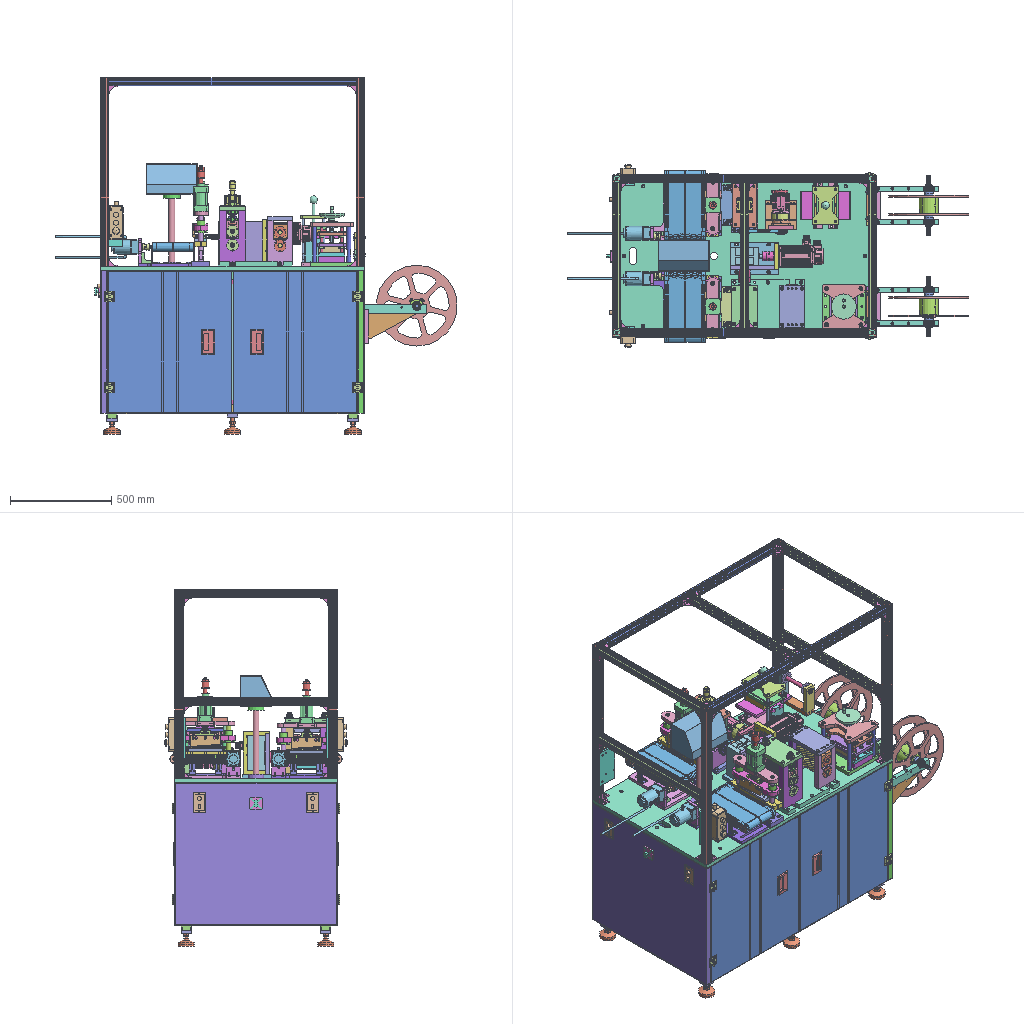Assembly | STEP file | 152 different items | 378 placed | box 1984 x 906 x 1760 mm
Parts list (item | name | quantity | parent item | size | volume):
1 | YBQDJ-FLJ-1 | x4 | in YBQDJ-FLJ | 400 x 8 x 400 mm | 566908 mm3
2 | YBQDJ-FLJ-3 | x2 | in YBQDJ-FLJ | - | -
3 | YBQDJ-FLJ-2 | x2 | in YBQDJ-FLJ | 95 x 103 x 95 mm | 482469 mm3
4 | YBQDJ-FLJ-5 | x2 | in YBQDJ-FLJ | 20 x 190 x 190 mm | 661776 mm3
5 | YBQDJ-FLJ-4 | x4 | in YBQDJ-FLJ | 310 x 25 x 45 mm | 300462 mm3
6 | YBQDJ-FLJ-6 | x4 | in YBQDJ-FLJ | 237.857 x 15 x 120 mm | 224363 mm3
7 | YBQDJ-FLJ-7 | x8 | in YBQDJ-FLJ | 15 x 33 x 33 mm | 11378 mm3
8 | YBQDJ-YL-1 | x1 | in YBQDJ-YL | 210 x 210 x 20 mm | 848713 mm3
9 | YBQDJ-YL-8 | x4 | in YBQDJ-YL | 12 x 12 x 182 mm | 19664 mm3
10 | YBQDJ-YL-13 | x2 | in YBQDJ-YL | 18.475 x 16 x 75 mm | 8074 mm3
11 | YBQDJ-YL-2 | x2 | in YBQDJ-YL | 130 x 30 x 30 mm | 104775 mm3
12 | YBQDJ-YL-10 | x1 | in YBQDJ-YL | 125 x 125 x 70 mm | 226936 mm3
13 | YBQDJ-YL-5 | x1 | in YBQDJ-YL | 140 x 220 x 15 mm | 360572 mm3
14 | YBQDJ-YL-9 | x4 | in YBQDJ-YL | 20 x 20 x 198 mm | 57396 mm3
15 | YBQDJ-YL-14 | x8 | in YBQDJ-YL | 32 x 32 x 30 mm | 10494 mm3
16 | YBQDJ-YL-12 | x1 | in YBQDJ-YL | 24.249 x 21 x 7 mm | 1795 mm3
17 | YBQDJ-YL-3 | x1 | in YBQDJ-YL | 130 x 210 x 15 mm | 393827 mm3
18 | YBQDJ-YL-7 | x1 | in YBQDJ-YL | 130 x 120 x 30 mm | 464984 mm3
19 | YBQDJ-YL-4 | x1 | in YBQDJ-YL | 140 x 220 x 15 mm | 408740 mm3
20 | YBQDJ-YL-11 | x1 | in YBQDJ-YL | 20 x 20 x 118 mm | 24858 mm3
21 | YBQDJ-YL-6 | x1 | in YBQDJ-YL | 210 x 220 x 20 mm | 625567 mm3
22 | YBQDJ-YL-15 | x2 | in YBQDJ-YL | 54 x 54 x 6 mm | 8414 mm3
23 | YBQDJ-YL-16 | x2 | in YBQDJ-YL | 32 x 32 x 9 mm | 3911 mm3
24 | YBQDJ-YL-17 | x1 | in YBQDJ-YL | 44 x 44 x 32 mm | 13018 mm3
25 | YBQDJ-YB-1 | x1 | in YBQDJ-YB | 360 x 270 x 24 mm | 2084097 mm3
26 | YBQDJ-YB-3 | x2 | in YBQDJ-YB | 80 x 30 x 70 mm | 107518 mm3
27 | YBQDJ-YB-18 | x1 | in YBQDJ-YB | 220 x 20 x 210 mm | 773333 mm3
28 | YBQDJ-YB-16 | x1 | in YBQDJ-YB | 33 x 210 x 33 mm | 88192 mm3
29 | YBQDJ-YB-17 | x1 | in YBQDJ-YB | 55 x 66 x 55 mm | 122440 mm3
30 | YBQDJ-YB-20 | x1 | in YBQDJ-YB | 193 x 155 x 174 mm | 2083887 mm3
31 | YBQDJ-YB-5 | x2 | in YBQDJ-YB | 68.992 x 218 x 68.953 mm | 543044 mm3
32 | YBQDJ-YB-6 | x1 | in YBQDJ-YB | 130 x 38 x 273 mm | 843391 mm3
33 | YBQDJ-YB-15 | x2 | in YBQDJ-YB | 69.832 x 130 x 69.818 mm | 396551 mm3
34 | YBQDJ-YB-8 | x2 | in YBQDJ-YB | 30 x 34.641 x 119.5 mm | 39653 mm3
35 | YBQDJ-YB-13 | x2 | in YBQDJ-YB | 59 x 10.5 x 59 mm | 15659 mm3
36 | YBQDJ-YB-12 | x2 | in YBQDJ-YB | 59 x 19 x 59 mm | 24092 mm3
37 | YBQDJ-YB-22 | x1 | in YBQDJ-YB | 275 x 158 x 110 mm | 3118501 mm3
38 | YBQDJ-YB-9 | x4 | in YBQDJ-YB | 50 x 50 x 14 mm | 18346 mm3
39 | YBQDJ-YB-7 | x2 | in YBQDJ-YB | 76 x 38 x 80 mm | 112101 mm3
40 | YBQDJ-YB-19 | x1 | in YBQDJ-YB | 240 x 160 x 19 mm | 686478 mm3
41 | YBQDJ-YB-21 | x1 | in YBQDJ-YB | 20 x 130 x 210 mm | 393461 mm3
42 | YBQDJ-YB-2 | x1 | in YBQDJ-YB | 120 x 30 x 223 mm | 466414 mm3
43 | YBQDJ-YB-11 | x1 | in YBQDJ-YB | 33 x 245 x 33 mm | 98573 mm3
44 | YBQDJ-YB-14 | x4 | in YBQDJ-YB | 59 x 5 x 59 mm | 11475 mm3
45 | YBQDJ-YB-4 | x1 | in YBQDJ-YB | 120 x 210 x 20 mm | 483124 mm3
46 | YBQDJ-YB-10 | x2 | in YBQDJ-YB | 42.8 x 42.8 x 20 mm | 13331 mm3
47 | YBQDJ-YB-23 | x1 | in YBQDJ-YB | 55 x 45 x 45 mm | 72571 mm3
48 | YBQDJ-YB-24 | x2 | in YBQDJ-YB | 30 x 10 x 30 mm | 3895 mm3
49 | YBQDJ-YB-25 | x1 | in YBQDJ-YB | - | -
50 | YBQDJ-YB-27 | x1 | in YBQDJ-YB | 130 x 38 x 273 mm | 843391 mm3
51 | YBQDJ-YB-26 | x1 | in YBQDJ-YB | 120 x 30 x 223 mm | 466414 mm3
52 | YBQDJ-YB-28 | x1 | in YBQDJ-YB | 130 x 210 x 20 mm | 518119 mm3
53 | YBQDJ-YB-29 | x16 | in YBQDJ-YB | 42 x 12 x 42 mm | 8686 mm3
54 | YBQDJ-YB-30 | x2 | in YBQDJ-YB | 34.5 x 10 x 4 mm | 1380 mm3
55 | YBQDJ-YB-34 | x1 | in YBQDJ-YB | 164.076 x 196 x 5.026 mm | 23129 mm3
56 | YBQDJ-YB-31 | x2 | in YBQDJ-YB | 40 x 30 x 80 mm | 9225 mm3
57 | YBQDJ-YB-32 | x1 | in YBQDJ-YB | 139.076 x 196 x 5.026 mm | 26086 mm3
58 | YBQDJ-YB-33 | x2 | in YBQDJ-YB | 20 x 20 x 4 mm | 942.478 mm3
59 | YBQDJ-QD-1 | x2 | in YBQDJ-QD-BD, YBQDJ-QD-PD | 90 x 300 x 25 mm | 495978 mm3
60 | YBQDJ-QD-7 | x4 | in YBQDJ-QD-BD, YBQDJ-QD-PD | 62 x 62 x 59 mm | 57722 mm3
61 | YBQDJ-QD-10 | x2 | in YBQDJ-QD-BD, YBQDJ-QD-PD | 75 x 290 x 20 mm | 318824 mm3
62 | YBQDJ-QD-4 | x2 | in YBQDJ-QD-BD, YBQDJ-QD-PD | 20 x 190 x 15 mm | 51822 mm3
63 | YBQDJ-QD-3 | x2 | in YBQDJ-QD-BD, YBQDJ-QD-PD | 60 x 310 x 25 mm | 397510 mm3
64 | YBQDJ-QD-2 | x2 | in YBQDJ-QD-BD | 25 x 25 x 254 mm | 111454 mm3
65 | YBQDJ-QD-11 | x2 | in YBQDJ-QD-BD, YBQDJ-QD-PD | 75 x 75 x 272 mm | 699847 mm3
66 | YBQDJ-QD-5 | x2 | in YBQDJ-QD-BD, YBQDJ-QD-PD | 35 x 190 x 15 mm | 92776 mm3
67 | YBQDJ-QD-8 | x2 | in YBQDJ-QD-BD, YBQDJ-QD-PD | 35 x 90 x 25 mm | 38677 mm3
68 | YBQDJ-QD-6 | x2 | in YBQDJ-QD-BD, YBQDJ-QD-PD | 70 x 300 x 25 mm | 414235 mm3
69 | YBQDJ-QD-9 | x2 | in YBQDJ-QD-BD, YBQDJ-QD-PD | 34 x 34 x 24 mm | 13509 mm3
70 | YBQDJ-QD-12 | x2 | in YBQDJ-QD-BD, YBQDJ-QD-PD | 10 x 150 x 65 mm | 69081 mm3
71 | YBQDJ-SSJ-1 | x1 | in YBQDJ-SSJ-BD | 280 x 320 x 15 mm | 982860 mm3
72 | YBQDJ-SSJ-8 | x2 | in YBQDJ-SSJ-BD, YBQD-SSJ-PD_MODEL | 50 x 20 x 50 mm | 24742 mm3
73 | YBQDJ-SSJ-7 | x2 | in YBQDJ-SSJ-BD, YBQD-SSJ-PD_MODEL | 227 x 40.957 x 41.285 mm | 212732 mm3
74 | YBQDJ-SSJ-3 | x2 | in YBQDJ-SSJ-BD, YBQD-SSJ-PD_MODEL | 200 x 350 x 44 mm | 311989 mm3
75 | YBQDJ-SSJ-11 | x2 | in YBQDJ-SSJ-BD, YBQD-SSJ-PD_MODEL | 35 x 30 x 30 mm | 20965 mm3
76 | YBQDJ-SSJ-9 | x2 | in YBQDJ-SSJ-BD, YBQD-SSJ-PD_MODEL | 15 x 70 x 120 mm | 105388 mm3
77 | YBQDJ-SSJ-6 | x2 | in YBQDJ-SSJ-BD, YBQD-SSJ-PD_MODEL | 196 x 40 x 40 mm | 211425 mm3
78 | YBQDJ-SSJ-4 | x8 | in YBQDJ-SSJ-BD, YBQD-SSJ-PD_MODEL | 20 x 85 x 39 mm | 27065 mm3
79 | YBQDJ-SSJ-10 | x2 | in YBQDJ-SSJ-BD, YBQD-SSJ-PD_MODEL | - | -
80 | YBQDJ-SSJ-2 | x8 | in YBQDJ-SSJ-BD, YBQD-SSJ-PD_MODEL | 40 x 30 x 80 mm | 9225 mm3
81 | YBQDJ-SSJ-5 | x4 | in YBQDJ-SSJ-BD, YBQD-SSJ-PD_MODEL | 20 x 215 x 40 mm | 63524 mm3
82 | YBQDJ-YY-1 | x1 | in YBQDJ-YY | 120 x 230 x 20 mm | 476492 mm3
83 | YBQDJ-YY-3 | x1 | in YBQDJ-YY | 80 x 20 x 148 mm | 197857 mm3
84 | YBQDJ-YY-5 | x1 | in YBQDJ-YY | 130 x 120 x 30 mm | 465920 mm3
85 | YBQDJ-YY-2 | x1 | in YBQDJ-YY | 80 x 20 x 148 mm | 197857 mm3
86 | YBQDJ-YY-7 | x1 | in YBQDJ-YY | 130 x 190 x 15 mm | 325427 mm3
87 | YBQDJ-YY-6 | x4 | in YBQDJ-YY | 32 x 32 x 30 mm | 10494 mm3
88 | YBQDJ-YY-10 | x4 | in YBQDJ-YY | 12 x 12 x 237 mm | 24995 mm3
89 | YBQDJ-YY-8 | x1 | in YBQDJ-YY | 130 x 190 x 15 mm | 272574 mm3
90 | YBQDJ-YY-4 | x1 | in YBQDJ-YY | 250 x 190 x 15 mm | 563148 mm3
91 | YBQDJ-YY-9 | x1 | in YBQDJ-YY | 40 x 40 x 166 mm | 52339 mm3
92 | YBQDJ-PD-1 | x1 | in YBQDJ-PD_MODEL | 150 x 140 x 20 mm | 385255 mm3
93 | YBQDJ-PD-4 | x2 | in YBQDJ-PD_MODEL | 67 x 28.5 x 67 mm | 55543 mm3
94 | YBQDJ-PD-7 | x1 | in YBQDJ-PD_MODEL | 130 x 29.2 x 127.5 mm | 362195 mm3
95 | YBQDJ-PD-3 | x1 | in YBQDJ-PD_MODEL | 120 x 20 x 138 mm | 191169 mm3
96 | YBQDJ-PD-5 | x1 | in YBQDJ-PD_MODEL | 245.482 x 15 x 95 mm | 17074 mm3
97 | YBQDJ-PD-9 | x1 | in YBQDJ-PD_MODEL | 68.992 x 253 x 68.953 mm | 537694 mm3
98 | YBQDJ-PD-8 | x1 | in YBQDJ-PD_MODEL | 130 x 29.2 x 127.5 mm | 362195 mm3
99 | YBQDJ-PD-11 | x4 | in YBQDJ-PD_MODEL | 32 x 32 x 57 mm | 16408 mm3
100 | YBQDJ-PD-10 | x1 | in YBQDJ-PD_MODEL | 68.992 x 218 x 68.953 mm | 532441 mm3
101 | YBQDJ-PD-6 | x1 | in YBQDJ-PD_MODEL | 130 x 270 x 19 mm | 640127 mm3
102 | YBQDJ-PD-2 | x1 | in YBQDJ-PD_MODEL | - | 675014 mm3
103 | YBQDJ-PD-16 | x1 | in YBQDJ-PD_MODEL | 34 x 34 x 24 mm | 12336 mm3
104 | YBQDJ-PD-15 | x1 | in YBQDJ-PD_MODEL | 76 x 84.5 x 162 mm | 333527 mm3
105 | YBQDJ-PD-17 | x1 | in YBQDJ-PD_MODEL | 35 x 90 x 25 mm | 38677 mm3
106 | YBQDJ-PD-13 | x4 | in YBQDJ-PD_MODEL | 12 x 12 x 284 mm | 30280 mm3
107 | YBQDJ-PD-14 | x1 | in YBQDJ-PD_MODEL | 120 x 220 x 20 mm | 489101 mm3
108 | YBQDJ-PD-18 | x1 | in YBQDJ-PD_MODEL | 40 x 220 x 15 mm | 117739 mm3
109 | YBQDJ-PD-19 | x4 | in YBQDJ-PD_MODEL | 53 x 13 x 53 mm | 13997 mm3
110 | YBQDJ-PD-12 | x2 | in YBQDJ-PD_MODEL | 130 x 29.2 x 80 mm | 97793 mm3
111 | YBQDJ-PD-20 | x8 | in YBQDJ-PD_MODEL | 35 x 11 x 35 mm | 5907 mm3
112 | YBQDJ-PD-21 | x1 | in YBQDJ-PD_MODEL | 31.177 x 27 x 9 mm | 3802 mm3
113 | YBQDJ-PD-24 | x2 | in YBQDJ-PD_MODEL | 20 x 20 x 4 mm | 1030 mm3
114 | YBQDJ-PD-25 | x2 | in YBQDJ-PD_MODEL | 40 x 30 x 80 mm | 9225 mm3
115 | YBQDJ-PD-22 | x1 | in YBQDJ-PD_MODEL | 139.076 x 196 x 5.026 mm | 26086 mm3
116 | YBQDJ-PD-23 | x1 | in YBQDJ-PD_MODEL | 164.076 x 196 x 5.026 mm | 23129 mm3
117 | YBQDJ-QD-PD-2 | x2 | in YBQDJ-QD-PD | 25 x 25 x 264 mm | 116363 mm3
118 | YBQDJ-SSJ-PD-1 | x1 | in YBQD-SSJ-PD_MODEL | 280 x 320 x 15 mm | 982860 mm3
119 | YBQDJ large plate | x1 | in Crimp-cut integrated machine, general type | 1300 x 800 x 20 mm | 20508106 mm3
120 | YBQDJ-DX-1 | x2 | in YBQDJ-DX-PD_MODEL, YBQDJ-DX-BD_MODEL | 50 x 200 x 20 mm | 177964 mm3
121 | YBQDJ-DX-3 | x4 | in YBQDJ-DX-PD_MODEL, YBQDJ-DX-BD_MODEL | 60 x 16 x 60 mm | 19587 mm3
122 | YBQDJ-DX-6 | x8 | in YBQDJ-DX-PD_MODEL, YBQDJ-DX-BD_MODEL | 32 x 10 x 32 mm | 4745 mm3
123 | YBQDJ-DX-4 | x2 | in YBQDJ-DX-PD_MODEL, YBQDJ-DX-BD_MODEL | 20 x 200 x 20 mm | 54352 mm3
124 | YBQDJ-DX-5 | x2 | in YBQDJ-DX-PD_MODEL, YBQDJ-DX-BD_MODEL | - | -
125 | YBQDJ-DX-2 | x1 | in YBQDJ-DX-PD_MODEL | 50 x 20 x 164 mm | 134384 mm3
126 | YBQDJ-DX-7 | x1 | in YBQDJ-DX-PD_MODEL | 50 x 20 x 164 mm | 134384 mm3
127 | YBQDJ-DX-BD-2 | x1 | in YBQDJ-DX-BD_MODEL | 50 x 20 x 79 mm | 49384 mm3
128 | YBQDJ-DX-BD-7 | x1 | in YBQDJ-DX-BD_MODEL | 50 x 20 x 79 mm | 49384 mm3
129 | 40x40-930 | x4 | in YBQDJ-LXC_MODEL | 40 x 40 x 930 mm | 513720 mm3
130 | 40x40-1220 | x2 | in YBQDJ-LXC_MODEL | 1220 x 40 x 40 mm | 673913 mm3
131 | 40x40-720 | x5 | in YBQDJ-LXC_MODEL | 40 x 720 x 40 mm | 397719 mm3
132 | 40x40 angle bracket | x28 | in YBQDJ-LXC_MODEL | 39.8 x 40 x 39.8 mm | 14360 mm3
133 | Button box plate | x2 | in YBQDJ-LXC_MODEL | 105 x 10 x 200 mm | 208063 mm3
134 | Button box | x2 | in YBQDJ-LXC_MODEL | 70 x 93 x 188 mm | 866675 mm3
135 | Touch screen assembly | x1 | in Crimp-cut integrated machine, general type | 250 x 150 x 505 mm | 675168 mm3
136 | 50x50x640 | x6 | in YBQDJ-JJ_MODEL | 50 x 640 x 50 mm | 562265 mm3
137 | 50x50x1240 | x2 | in YBQDJ-JJ_MODEL | 1240 x 50 x 50 mm | 1089389 mm3
138 | Foot cup | x6 | in 50x50x680_MODEL, 50x50x1140_MODEL | 80 x 80 x 135 mm | 154518 mm3
139 | Spacer block | x6 | in 50x50x680_MODEL, 50x50x1140_MODEL | 50 x 50 x 15 mm | 35145 mm3
140 | SOLID | x4 | in 50x50x680_MODEL | 50 x 50 x 680 mm | 597407 mm3
141 | Door magnet catch | x4 | in 50x50x610_MODEL | 40 x 5 x 20 mm | 3632 mm3
142 | SOLID | x2 | in 50x50x610_MODEL | 50 x 50 x 610 mm | 535909 mm3
143 | SOLID | x2 | in 50x50x1140_MODEL | 1140 x 50 x 50 mm | 1000530 mm3
144 | Crossbeam | x2 | in YBQDJ-JJ_MODEL | 15 x 730 x 50 mm | 541334 mm3
145 | Reinforcing rib | x4 | in YBQDJ-BJ-1_MODEL | 80 x 26.7 x 696 mm | 106400 mm3
146 | Handle | x4 | in YBQDJ-BJ-1_MODEL | 69 x 21 x 119 mm | 44051 mm3
147 | SOLID | x4 | in YBQDJ-BJ-1_MODEL | 615 x 30 x 705 mm | 627775 mm3
148 | Hinge | x8 | in YBQDJ-BJ_MODEL | 50 x 12.7 x 49.8 mm | 17221 mm3
149 | Power switch | x1 | in YBQDJ-BJ-2_MODEL | 64 x 60 x 60 mm | 180692 mm3
150 | Speed control panel | x2 | in YBQDJ-BJ-2_MODEL | 122.5 x 60 x 100 mm | 404808 mm3
151 | SOLID | x1 | in YBQDJ-BJ-2_MODEL | 55 x 800 x 705 mm | 825706 mm3
152 | YBQDJ-BJ-3 | x1 | in YBQDJ-BJ_MODEL | 55 x 800 x 705 mm | 823970 mm3
Placements (level | parent | child | x y z in mm | rotation matrix by rows), first 330 of 406 lines:
1 | Crimp-cut integrated machine, general type | YBQDJ-FLJ | 0.0 0.0 0.0 | 1 0 0 0 1 0 0 0 1
2 | YBQDJ-FLJ | YBQDJ-FLJ-1 | 0.0 0.0 0.0 | 1 0 0 0 1 0 0 0 1
2 | YBQDJ-FLJ | YBQDJ-FLJ-3 | 0.0 0.0 0.0 | 1 0 0 0 1 0 0 0 1
2 | YBQDJ-FLJ | YBQDJ-FLJ-2 | 0.0 0.0 0.0 | 1 0 0 0 1 0 0 0 1
2 | YBQDJ-FLJ | YBQDJ-FLJ-1 | 0.0 91.0 0.0 | 1 0 0 0 1 0 0 0 1
2 | YBQDJ-FLJ | YBQDJ-FLJ-5 | 0.0 0.0 0.0 | 1 0 0 0 1 0 0 0 1
2 | YBQDJ-FLJ | YBQDJ-FLJ-4 | 0.0 0.0 0.0 | 1 0 0 0 1 0 0 0 1
2 | YBQDJ-FLJ | YBQDJ-FLJ-6 | 0.0 0.0 0.0 | 1 0 0 0 1 0 0 0 1
2 | YBQDJ-FLJ | YBQDJ-FLJ-6 | 0.0 165.0 0.0 | 1 0 0 0 1 0 0 0 1
2 | YBQDJ-FLJ | YBQDJ-FLJ-4 | 0.0 165.0 0.0 | 1 0 0 0 1 0 0 0 1
2 | YBQDJ-FLJ | YBQDJ-FLJ-7 | -0.0 90.0 -140.0 | 1 0 0 0 1 0 0 0 1
2 | YBQDJ-FLJ | YBQDJ-FLJ-7 | -0.0 90.0 -0.0 | 1 0 0 0 1 0 0 0 1
2 | YBQDJ-FLJ | YBQDJ-FLJ-7 | 0.0 0.0 0.0 | 1 0 0 0 1 0 0 0 1
2 | YBQDJ-FLJ | YBQDJ-FLJ-7 | 0.0 0.0 -140.0 | 1 0 0 0 1 0 0 0 1
1 | Crimp-cut integrated machine, general type | YBQDJ-FLJ | 0.0 500.0 0.0 | 1 0 0 0 1 0 0 0 1
2 | YBQDJ-FLJ | YBQDJ-FLJ-1 | 0.0 0.0 0.0 | 1 0 0 0 1 0 0 0 1
2 | YBQDJ-FLJ | YBQDJ-FLJ-3 | 0.0 0.0 0.0 | 1 0 0 0 1 0 0 0 1
2 | YBQDJ-FLJ | YBQDJ-FLJ-2 | 0.0 0.0 0.0 | 1 0 0 0 1 0 0 0 1
2 | YBQDJ-FLJ | YBQDJ-FLJ-1 | 0.0 91.0 0.0 | 1 0 0 0 1 0 0 0 1
2 | YBQDJ-FLJ | YBQDJ-FLJ-5 | 0.0 0.0 0.0 | 1 0 0 0 1 0 0 0 1
2 | YBQDJ-FLJ | YBQDJ-FLJ-4 | 0.0 0.0 0.0 | 1 0 0 0 1 0 0 0 1
2 | YBQDJ-FLJ | YBQDJ-FLJ-6 | 0.0 0.0 0.0 | 1 0 0 0 1 0 0 0 1
2 | YBQDJ-FLJ | YBQDJ-FLJ-6 | 0.0 165.0 0.0 | 1 0 0 0 1 0 0 0 1
2 | YBQDJ-FLJ | YBQDJ-FLJ-4 | 0.0 165.0 0.0 | 1 0 0 0 1 0 0 0 1
2 | YBQDJ-FLJ | YBQDJ-FLJ-7 | -0.0 90.0 -140.0 | 1 0 0 0 1 0 0 0 1
2 | YBQDJ-FLJ | YBQDJ-FLJ-7 | -0.0 90.0 -0.0 | 1 0 0 0 1 0 0 0 1
2 | YBQDJ-FLJ | YBQDJ-FLJ-7 | 0.0 0.0 0.0 | 1 0 0 0 1 0 0 0 1
2 | YBQDJ-FLJ | YBQDJ-FLJ-7 | 0.0 0.0 -140.0 | 1 0 0 0 1 0 0 0 1
1 | Crimp-cut integrated machine, general type | YBQDJ-YL | 0.0 0.0 0.0 | 1 0 0 0 1 0 0 0 1
2 | YBQDJ-YL | YBQDJ-YL-1 | 0.0 0.0 0.0 | 1 0 0 0 1 0 0 0 1
2 | YBQDJ-YL | YBQDJ-YL-8 | 0.0 0.0 0.0 | 1 0 0 0 1 0 0 0 1
2 | YBQDJ-YL | YBQDJ-YL-13 | 0.0 0.0 0.0 | 1 0 0 0 1 0 0 0 1
2 | YBQDJ-YL | YBQDJ-YL-2 | 0.0 0.0 0.0 | 1 0 0 0 1 0 0 0 1
2 | YBQDJ-YL | YBQDJ-YL-10 | 0.0 0.0 0.0 | 1 0 0 0 1 0 0 0 1
2 | YBQDJ-YL | YBQDJ-YL-5 | 0.0 0.0 0.0 | 1 0 0 0 1 0 0 0 1
2 | YBQDJ-YL | YBQDJ-YL-9 | 0.0 0.0 0.0 | 1 0 0 0 1 0 0 0 1
2 | YBQDJ-YL | YBQDJ-YL-14 | 0.0 0.0 0.0 | 1 0 0 0 1 0 0 0 1
2 | YBQDJ-YL | YBQDJ-YL-12 | 0.0 0.0 0.5 | 1 0 0 0 1 0 0 0 1
2 | YBQDJ-YL | YBQDJ-YL-3 | 0.0 0.0 0.0 | 1 0 0 0 1 0 0 0 1
2 | YBQDJ-YL | YBQDJ-YL-7 | 0.0 0.0 0.0 | 1 0 0 0 1 0 0 0 1
2 | YBQDJ-YL | YBQDJ-YL-4 | 0.0 0.0 0.0 | 1 0 0 0 1 0 0 0 1
2 | YBQDJ-YL | YBQDJ-YL-11 | 0.0 0.0 0.0 | 1 0 0 0 1 0 0 0 1
2 | YBQDJ-YL | YBQDJ-YL-6 | 0.0 0.0 0.0 | 1 0 0 0 1 0 0 0 1
2 | YBQDJ-YL | YBQDJ-YL-2 | 0.0 180.0 0.0 | 1 0 0 0 1 0 0 0 1
2 | YBQDJ-YL | YBQDJ-YL-14 | 100.0 0.0 0.0 | 1 0 0 0 1 0 0 0 1
2 | YBQDJ-YL | YBQDJ-YL-14 | 100.0 180.0 0.0 | 1 0 0 0 1 0 0 0 1
2 | YBQDJ-YL | YBQDJ-YL-14 | 0.0 180.0 0.0 | 1 0 0 0 1 0 0 0 1
2 | YBQDJ-YL | YBQDJ-YL-14 | 613.0 0.0 260.0 | -1 0 0 0 1 0 0 0 -1
2 | YBQDJ-YL | YBQDJ-YL-14 | 513.0 0.0 260.0 | -1 0 0 0 1 0 0 0 -1
2 | YBQDJ-YL | YBQDJ-YL-14 | 613.0 180.0 260.0 | -1 0 0 0 1 0 0 0 -1
2 | YBQDJ-YL | YBQDJ-YL-14 | 513.0 180.0 260.0 | -1 0 0 0 1 0 0 0 -1
2 | YBQDJ-YL | YBQDJ-YL-13 | 0.0 180.0 0.0 | 1 0 0 0 1 0 0 0 1
2 | YBQDJ-YL | YBQDJ-YL-8 | 100.0 0.0 0.0 | 1 0 0 0 1 0 0 0 1
2 | YBQDJ-YL | YBQDJ-YL-8 | 0.0 180.0 0.0 | 1 0 0 0 1 0 0 0 1
2 | YBQDJ-YL | YBQDJ-YL-8 | 100.0 180.0 0.0 | 1 0 0 0 1 0 0 0 1
2 | YBQDJ-YL | YBQDJ-YL-9 | 170.0 0.0 0.0 | 1 0 0 0 1 0 0 0 1
2 | YBQDJ-YL | YBQDJ-YL-9 | 170.0 180.0 0.0 | 1 0 0 0 1 0 0 0 1
2 | YBQDJ-YL | YBQDJ-YL-9 | 0.0 180.0 0.0 | 1 0 0 0 1 0 0 0 1
2 | YBQDJ-YL | YBQDJ-YL-15 | 0.0 0.0 0.0 | 1 0 0 0 1 0 0 0 1
2 | YBQDJ-YL | YBQDJ-YL-16 | 0.0 0.0 0.0 | 1 0 0 0 1 0 0 0 1
2 | YBQDJ-YL | YBQDJ-YL-17 | 0.0 0.0 0.0 | 1 0 0 0 1 0 0 0 1
2 | YBQDJ-YL | YBQDJ-YL-16 | 0.0 0.0 9.0 | 1 0 0 0 1 0 0 0 1
2 | YBQDJ-YL | YBQDJ-YL-15 | 613.0 0.0 408.0 | -1 0 0 0 1 0 0 0 -1
1 | Crimp-cut integrated machine, general type | YBQDJ-YB | 0.0 0.0 0.0 | 1 0 0 0 1 0 0 0 1
2 | YBQDJ-YB | YBQDJ-YB-1 | 0.0 0.0 0.0 | 1 0 0 0 1 0 0 0 1
2 | YBQDJ-YB | YBQDJ-YB-3 | 0.0 0.0 0.0 | 1 0 0 0 1 0 0 0 1
2 | YBQDJ-YB | YBQDJ-YB-18 | 0.0 0.0 0.0 | 1 0 0 0 1 0 0 0 1
2 | YBQDJ-YB | YBQDJ-YB-16 | 0.0 0.0 0.0 | 1 0 0 0 1 0 0 0 1
2 | YBQDJ-YB | YBQDJ-YB-17 | 0.0 0.0 0.0 | 1 0 0 0 1 0 0 0 1
2 | YBQDJ-YB | YBQDJ-YB-20 | 0.0 0.0 0.0 | 1 0 0 0 1 0 0 0 1
2 | YBQDJ-YB | YBQDJ-YB-5 | 0.0 0.0 0.0 | 1 0 0 0 1 0 0 0 1
2 | YBQDJ-YB | YBQDJ-YB-6 | 0.0 0.0 0.0 | 1 0 0 0 1 0 0 0 1
2 | YBQDJ-YB | YBQDJ-YB-15 | 0.0 0.0 0.0 | 1 0 0 0 1 0 0 0 1
2 | YBQDJ-YB | YBQDJ-YB-8 | 0.0 0.0 0.0 | 1 0 0 0 1 0 0 0 1
2 | YBQDJ-YB | YBQDJ-YB-13 | 0.0 0.0 0.0 | 1 0 0 0 1 0 0 0 1
2 | YBQDJ-YB | YBQDJ-YB-12 | 0.0 0.0 0.0 | 1 0 0 0 1 0 0 0 1
2 | YBQDJ-YB | YBQDJ-YB-22 | 0.0 0.0 0.0 | 1 0 0 0 1 0 0 0 1
2 | YBQDJ-YB | YBQDJ-YB-9 | 0.0 0.0 0.0 | 1 0 0 0 1 0 0 0 1
2 | YBQDJ-YB | YBQDJ-YB-7 | 0.0 0.0 0.0 | 1 0 0 0 1 0 0 0 1
2 | YBQDJ-YB | YBQDJ-YB-19 | 0.0 0.0 0.0 | 1 0 0 0 1 0 0 0 1
2 | YBQDJ-YB | YBQDJ-YB-21 | 0.0 0.0 0.0 | 1 0 0 0 1 0 0 0 1
2 | YBQDJ-YB | YBQDJ-YB-2 | 0.0 0.0 0.0 | 1 0 0 0 1 0 0 0 1
2 | YBQDJ-YB | YBQDJ-YB-11 | 0.0 0.0 0.0 | 1 0 0 0 1 0 0 0 1
2 | YBQDJ-YB | YBQDJ-YB-14 | 0.0 0.0 0.0 | 1 0 0 0 1 0 0 0 1
2 | YBQDJ-YB | YBQDJ-YB-4 | 0.0 0.0 0.0 | 1 0 0 0 1 0 0 0 1
2 | YBQDJ-YB | YBQDJ-YB-10 | 0.0 0.0 0.0 | 1 0 0 0 1 0 0 0 1
2 | YBQDJ-YB | YBQDJ-YB-23 | 0.0 0.0 0.0 | 1 0 0 0 1 0 0 0 1
2 | YBQDJ-YB | YBQDJ-YB-24 | 0.0 0.0 0.0 | 1 0 0 0 1 0 0 0 1
2 | YBQDJ-YB | YBQDJ-YB-25 | 0.0 0.0 0.0 | 1 0 0 0 1 0 0 0 1
2 | YBQDJ-YB | YBQDJ-YB-27 | 0.0 0.0 0.0 | 1 0 0 0 1 0 0 0 1
2 | YBQDJ-YB | YBQDJ-YB-26 | 0.0 0.0 0.0 | 1 0 0 0 1 0 0 0 1
2 | YBQDJ-YB | YBQDJ-YB-28 | 0.0 0.0 0.0 | 1 0 0 0 1 0 0 0 1
2 | YBQDJ-YB | YBQDJ-YB-29 | 0.0 0.0 0.0 | 1 0 0 0 1 0 0 0 1
2 | YBQDJ-YB | YBQDJ-YB-29 | 0.0 -12.0 0.0 | 1 0 0 0 1 0 0 0 1
2 | YBQDJ-YB | YBQDJ-YB-29 | 0.0 182.0 0.0 | 1 0 0 0 1 0 0 0 1
2 | YBQDJ-YB | YBQDJ-YB-29 | 0.0 170.0 0.0 | 1 0 0 0 1 0 0 0 1
2 | YBQDJ-YB | YBQDJ-YB-29 | 0.0 0.0 67.0 | 1 0 0 0 1 0 0 0 1
2 | YBQDJ-YB | YBQDJ-YB-29 | 0.0 170.0 67.0 | 1 0 0 0 1 0 0 0 1
2 | YBQDJ-YB | YBQDJ-YB-29 | 0.0 182.0 67.0 | 1 0 0 0 1 0 0 0 1
2 | YBQDJ-YB | YBQDJ-YB-5 | 0.0 0.0 67.0 | 1 0 0 0 1 0 0 0 1
2 | YBQDJ-YB | YBQDJ-YB-29 | 0.0 -12.0 67.0 | 1 0 0 0 1 0 0 0 1
2 | YBQDJ-YB | YBQDJ-YB-14 | -0.0 0.0 67.0 | 1 0 0 0 1 0 0 0 1
2 | YBQDJ-YB | YBQDJ-YB-3 | 103.0 -390.0 0.0 | -1 0 0 0 -1 0 0 0 1
2 | YBQDJ-YB | YBQDJ-YB-14 | 103.0 -390.0 0.0 | -1 0 0 0 -1 0 0 0 1
2 | YBQDJ-YB | YBQDJ-YB-14 | 103.0 -390.0 67.0 | -1 0 0 0 -1 0 0 0 1
2 | YBQDJ-YB | YBQDJ-YB-15 | 0.0 0.0 68.3 | 1 0 0 0 1 0 0 0 1
2 | YBQDJ-YB | YBQDJ-YB-29 | -235.0 12.0 3.0 | 1 0 0 0 1 0 0 0 1
2 | YBQDJ-YB | YBQDJ-YB-29 | -235.0 0.0 3.0 | 1 0 0 0 1 0 0 0 1
2 | YBQDJ-YB | YBQDJ-YB-29 | -235.0 0.0 71.3 | 1 0 0 0 1 0 0 0 1
2 | YBQDJ-YB | YBQDJ-YB-29 | -235.0 12.0 71.3 | 1 0 0 0 1 0 0 0 1
2 | YBQDJ-YB | YBQDJ-YB-12 | -0.0 0.0 68.3 | 1 0 0 0 1 0 0 0 1
2 | YBQDJ-YB | YBQDJ-YB-9 | 0.0 0.0 36.7 | 1 0 0 0 1 0 0 0 1
2 | YBQDJ-YB | YBQDJ-YB-7 | -367 -390 -0.0 | -1 1e-06 0 -1e-06 -1 0 0 0 1
2 | YBQDJ-YB | YBQDJ-YB-9 | 0.0 172.0 36.7 | 1 0 0 0 1 0 0 0 1
2 | YBQDJ-YB | YBQDJ-YB-8 | 0.0 172.0 0.0 | 1 0 0 0 1 0 0 0 1
2 | YBQDJ-YB | YBQDJ-YB-9 | 0.0 172.0 0.0 | 1 0 0 0 1 0 0 0 1
2 | YBQDJ-YB | YBQDJ-YB-10 | 0.0 172.0 0.0 | 1 0 0 0 1 0 0 0 1
2 | YBQDJ-YB | YBQDJ-YB-24 | 0.0 0.0 68.3 | 1 0 0 0 1 0 0 0 1
2 | YBQDJ-YB | YBQDJ-YB-29 | -235.0 166.5 3.0 | 1 0 0 0 1 0 0 0 1
2 | YBQDJ-YB | YBQDJ-YB-29 | -235.0 178.5 3.0 | 1 0 0 0 1 0 0 0 1
2 | YBQDJ-YB | YBQDJ-YB-13 | 0.0 0.0 68.3 | 1 0 0 0 1 0 0 0 1
2 | YBQDJ-YB | YBQDJ-YB-29 | -235.0 178.5 71.3 | 1 0 0 0 1 0 0 0 1
2 | YBQDJ-YB | YBQDJ-YB-29 | -235.0 166.5 71.3 | 1 0 0 0 1 0 0 0 1
2 | YBQDJ-YB | YBQDJ-YB-30 | 0.0 172.0 0.0 | 1 0 0 0 1 0 0 0 1
2 | YBQDJ-YB | YBQDJ-YB-30 | 0.0 0.0 0.0 | 1 0 0 0 1 0 0 0 1
2 | YBQDJ-YB | YBQDJ-YB-34 | 0.0 0.0 0.0 | 1 0 0 0 1 0 0 0 1
2 | YBQDJ-YB | YBQDJ-YB-31 | 0.0 0.0 0.0 | 1 0 0 0 1 0 0 0 1
2 | YBQDJ-YB | YBQDJ-YB-32 | -0.5 0.0 0.0 | 1 0 0 0 1 0 0 0 1
2 | YBQDJ-YB | YBQDJ-YB-33 | 0.0 0.0 0.0 | 1 0 0 0 1 0 0 0 1
2 | YBQDJ-YB | YBQDJ-YB-31 | 0.0 172.0 0.0 | 1 0 0 0 1 0 0 0 1
2 | YBQDJ-YB | YBQDJ-YB-33 | 0.0 172.0 0.0 | 1 0 0 0 1 0 0 0 1
1 | Crimp-cut integrated machine, general type | YBQDJ-QD-BD | 0.0 0.0 0.0 | 1 0 0 0 1 0 0 0 1
2 | YBQDJ-QD-BD | YBQDJ-QD-1 | 0.0 0.0 0.0 | 1 0 0 0 1 0 0 0 1
2 | YBQDJ-QD-BD | YBQDJ-QD-7 | 0.0 0.0 0.0 | 1 0 0 0 1 0 0 0 1
2 | YBQDJ-QD-BD | YBQDJ-QD-10 | 0.0 0.0 0.0 | 1 0 0 0 1 0 0 0 1
2 | YBQDJ-QD-BD | YBQDJ-QD-4 | 0.0 0.0 0.0 | 1 0 0 0 1 0 0 0 1
2 | YBQDJ-QD-BD | YBQDJ-QD-3 | 0.0 0.0 0.0 | 1 0 0 0 1 0 0 0 1
2 | YBQDJ-QD-BD | YBQDJ-QD-2 | 0.0 0.0 0.0 | 1 0 0 0 1 0 0 0 1
2 | YBQDJ-QD-BD | YBQDJ-QD-11 | 0.0 0.0 0.0 | 1 0 0 0 1 0 0 0 1
2 | YBQDJ-QD-BD | YBQDJ-QD-5 | 0.0 0.0 0.0 | 1 0 0 0 1 0 0 0 1
2 | YBQDJ-QD-BD | YBQDJ-QD-8 | 0.0 0.0 0.0 | 1 0 0 0 1 0 0 0 1
2 | YBQDJ-QD-BD | YBQDJ-QD-6 | 0.0 0.0 0.0 | 1 0 0 0 1 0 0 0 1
2 | YBQDJ-QD-BD | YBQDJ-QD-9 | 0.0 0.0 0.0 | 1 0 0 0 1 0 0 0 1
2 | YBQDJ-QD-BD | YBQDJ-QD-12 | 0.0 0.0 0.0 | 1 0 0 0 1 0 0 0 1
2 | YBQDJ-QD-BD | YBQDJ-QD-2 | 0.0 230.0 0.0 | 1 0 0 0 1 0 0 0 1
2 | YBQDJ-QD-BD | YBQDJ-QD-7 | 0.0 230.0 0.0 | 1 0 0 0 1 0 0 0 1
1 | Crimp-cut integrated machine, general type | YBQDJ-SSJ-BD | 0.0 0.0 0.0 | 1 0 0 0 1 0 0 0 1
2 | YBQDJ-SSJ-BD | YBQDJ-SSJ-1 | 0.0 0.0 0.0 | 1 0 0 0 1 0 0 0 1
2 | YBQDJ-SSJ-BD | YBQDJ-SSJ-8 | 0.0 0.0 0.0 | 1 0 0 0 1 0 0 0 1
2 | YBQDJ-SSJ-BD | YBQDJ-SSJ-7 | 0.0 0.0 0.0 | 1 0 0 0 1 0 0 0 1
2 | YBQDJ-SSJ-BD | YBQDJ-SSJ-3 | 0.0 0.0 0.0 | 1 0 0 0 1 0 0 0 1
2 | YBQDJ-SSJ-BD | YBQDJ-SSJ-11 | 0.0 0.0 0.0 | 1 0 0 0 1 0 0 0 1
2 | YBQDJ-SSJ-BD | YBQDJ-SSJ-9 | 0.0 0.0 0.0 | 1 0 0 0 1 0 0 0 1
2 | YBQDJ-SSJ-BD | YBQDJ-SSJ-6 | 0.0 0.0 0.0 | 1 0 0 0 1 0 0 0 1
2 | YBQDJ-SSJ-BD | YBQDJ-SSJ-4 | 0.0 0.0 0.0 | 1 0 0 0 1 0 0 0 1
2 | YBQDJ-SSJ-BD | YBQDJ-SSJ-10 | 0.0 0.0 0.0 | 1 0 0 0 1 0 0 0 1
2 | YBQDJ-SSJ-BD | YBQDJ-SSJ-2 | 0.0 0.0 0.0 | 1 0 0 0 1 0 0 0 1
2 | YBQDJ-SSJ-BD | YBQDJ-SSJ-4 | -0.0 -390.0 189.0 | 1 0 0 0 -1 0 0 0 -1
2 | YBQDJ-SSJ-BD | YBQDJ-SSJ-4 | -955.0 -390.0 -0.0 | -1 0 0 0 -1 0 0 0 1
2 | YBQDJ-SSJ-BD | YBQDJ-SSJ-4 | -955.0 0.0 189.0 | -1 0 0 0 1 0 0 0 -1
2 | YBQDJ-SSJ-BD | YBQDJ-SSJ-2 | 0.0 130.0 0.0 | 1 0 0 0 1 0 0 0 1
2 | YBQDJ-SSJ-BD | YBQDJ-SSJ-2 | -955.0 -520.0 0.0 | -1 0 0 0 -1 0 0 0 1
2 | YBQDJ-SSJ-BD | YBQDJ-SSJ-2 | -955.0 -390.0 0.0 | -1 0 0 0 -1 0 0 0 1
2 | YBQDJ-SSJ-BD | YBQDJ-SSJ-5 | -955.0 0.0 189.0 | -1 0 0 0 1 0 0 0 -1
2 | YBQDJ-SSJ-BD | YBQDJ-SSJ-5 | 0.0 0.0 0.0 | 1 0 0 0 1 0 0 0 1
1 | Crimp-cut integrated machine, general type | YBQDJ-YY | 0.0 0.0 0.0 | 1 0 0 0 1 0 0 0 1
2 | YBQDJ-YY | YBQDJ-YY-1 | 0.0 0.0 0.0 | 1 0 0 0 1 0 0 0 1
2 | YBQDJ-YY | YBQDJ-YY-3 | 0.0 0.0 0.0 | 1 0 0 0 1 0 0 0 1
2 | YBQDJ-YY | YBQDJ-YY-5 | 0.0 0.0 0.0 | 1 0 0 0 1 0 0 0 1
2 | YBQDJ-YY | YBQDJ-YY-2 | 0.0 0.0 0.0 | 1 0 0 0 1 0 0 0 1
2 | YBQDJ-YY | YBQDJ-YY-7 | 0.0 0.0 0.0 | 1 0 0 0 1 0 0 0 1
2 | YBQDJ-YY | YBQDJ-YY-6 | 0.0 0.0 0.0 | 1 0 0 0 1 0 0 0 1
2 | YBQDJ-YY | YBQDJ-YY-10 | 0.0 0.0 0.0 | 1 0 0 0 1 0 0 0 1
2 | YBQDJ-YY | YBQDJ-YY-8 | 0.0 0.0 0.0 | 1 0 0 0 1 0 0 0 1
2 | YBQDJ-YY | YBQDJ-YY-4 | 0.0 0.0 0.0 | 1 0 0 0 1 0 0 0 1
2 | YBQDJ-YY | YBQDJ-YY-9 | 0.0 0.0 0.0 | 1 0 0 0 1 0 0 0 1
2 | YBQDJ-YY | YBQDJ-YY-10 | 0.0 -160.0 0.0 | 1 0 0 0 1 0 0 0 1
2 | YBQDJ-YY | YBQDJ-YY-6 | 0.0 -160.0 0.0 | 1 0 0 0 1 0 0 0 1
2 | YBQDJ-YY | YBQDJ-YY-10 | -100.0 -160.0 0.0 | 1 0 0 0 1 0 0 0 1
2 | YBQDJ-YY | YBQDJ-YY-6 | -100.0 -160.0 0.0 | 1 0 0 0 1 0 0 0 1
2 | YBQDJ-YY | YBQDJ-YY-6 | -100.0 0.0 0.0 | 1 0 0 0 1 0 0 0 1
2 | YBQDJ-YY | YBQDJ-YY-10 | -100.0 0.0 0.0 | 1 0 0 0 1 0 0 0 1
1 | Crimp-cut integrated machine, general type | YBQDJ-PD_MODEL | 0.0 0.0 0.0 | 1 0 0 0 1 0 0 0 1
2 | YBQDJ-PD_MODEL | YBQDJ-PD-1 | 0.0 0.0 0.0 | 1 0 0 0 1 0 0 0 1
2 | YBQDJ-PD_MODEL | YBQDJ-PD-4 | 0.0 0.0 0.0 | 1 0 0 0 1 0 0 0 1
2 | YBQDJ-PD_MODEL | YBQDJ-PD-7 | 0.0 0.0 0.0 | 1 0 0 0 1 0 0 0 1
2 | YBQDJ-PD_MODEL | YBQDJ-PD-3 | 0.0 0.0 0.0 | 1 0 0 0 1 0 0 0 1
2 | YBQDJ-PD_MODEL | YBQDJ-PD-5 | 0.0 0.0 0.0 | 1 0 0 0 1 0 0 0 1
2 | YBQDJ-PD_MODEL | YBQDJ-PD-9 | 0.0 0.0 0.0 | 1 0 0 0 1 0 0 0 1
2 | YBQDJ-PD_MODEL | YBQDJ-PD-8 | 0.0 0.0 0.0 | 1 0 0 0 1 0 0 0 1
2 | YBQDJ-PD_MODEL | YBQDJ-PD-11 | 0.0 0.0 7.5 | 1 0 0 0 1 0 0 0 1
2 | YBQDJ-PD_MODEL | YBQDJ-PD-10 | 0.0 0.0 7.5 | 1 0 0 0 1 0 0 0 1
2 | YBQDJ-PD_MODEL | YBQDJ-PD-6 | 0.0 0.0 0.0 | 1 0 0 0 1 0 0 0 1
2 | YBQDJ-PD_MODEL | YBQDJ-PD-2 | 0.0 0.0 0.0 | 1 0 0 0 1 0 0 0 1
2 | YBQDJ-PD_MODEL | YBQDJ-PD-16 | 0.0 0.0 0.0 | 1 0 0 0 1 0 0 0 1
2 | YBQDJ-PD_MODEL | YBQDJ-PD-15 | 0.0 0.0 0.0 | 1 0 0 0 1 0 0 0 1
2 | YBQDJ-PD_MODEL | YBQDJ-PD-17 | 0.0 0.0 0.0 | 1 0 0 0 1 0 0 0 1
2 | YBQDJ-PD_MODEL | YBQDJ-PD-13 | 0.0 0.0 0.0 | 1 0 0 0 1 0 0 0 1
2 | YBQDJ-PD_MODEL | YBQDJ-PD-14 | 0.0 0.0 0.0 | 1 0 0 0 1 0 0 0 1
2 | YBQDJ-PD_MODEL | YBQDJ-PD-18 | 0.0 0.0 7.5 | 1 0 0 0 1 0 0 0 1
2 | YBQDJ-PD_MODEL | YBQDJ-PD-19 | 0.0 -0.4 0.0 | 1 0 0 0 1 0 0 0 1
2 | YBQDJ-PD_MODEL | YBQDJ-PD-12 | 0.0 0.0 7.5 | 1 0 0 0 1 0 0 0 1
2 | YBQDJ-PD_MODEL | YBQDJ-PD-20 | 0.0 0.0 0.0 | 1 0 0 0 1 0 0 0 1
2 | YBQDJ-PD_MODEL | YBQDJ-PD-20 | 0.0 11.0 0.0 | 1 0 0 0 1 0 0 0 1
2 | YBQDJ-PD_MODEL | YBQDJ-PD-19 | 0.0 -0.4 74.5 | 1 0 0 0 1 0 0 0 1
2 | YBQDJ-PD_MODEL | YBQDJ-PD-20 | 0.0 -0.0 74.5 | 1 0 0 0 1 0 0 0 1
2 | YBQDJ-PD_MODEL | YBQDJ-PD-20 | 0.0 11.0 74.5 | 1 0 0 0 1 0 0 0 1
2 | YBQDJ-PD_MODEL | YBQDJ-PD-19 | -367.0 610.4 0.0 | -1 0 0 0 -1 0 0 0 1
2 | YBQDJ-PD_MODEL | YBQDJ-PD-19 | -367.0 610.4 74.5 | -1 0 0 0 -1 0 0 0 1
2 | YBQDJ-PD_MODEL | YBQDJ-PD-12 | 0.0 -190.0 7.5 | 1 0 0 0 1 0 0 0 1
2 | YBQDJ-PD_MODEL | YBQDJ-PD-13 | 0.0 -190.0 0.0 | 1 0 0 0 1 0 0 0 1
2 | YBQDJ-PD_MODEL | YBQDJ-PD-11 | 0.0 -190.0 7.5 | 1 0 0 0 1 0 0 0 1
2 | YBQDJ-PD_MODEL | YBQDJ-PD-13 | -90.0 -190.0 0.0 | 1 0 0 0 1 0 0 0 1
2 | YBQDJ-PD_MODEL | YBQDJ-PD-11 | -90.0 -190.0 7.5 | 1 0 0 0 1 0 0 0 1
2 | YBQDJ-PD_MODEL | YBQDJ-PD-13 | -90.0 0.0 0.0 | 1 0 0 0 1 0 0 0 1
2 | YBQDJ-PD_MODEL | YBQDJ-PD-11 | -90.0 0.0 7.5 | 1 0 0 0 1 0 0 0 1
2 | YBQDJ-PD_MODEL | YBQDJ-PD-4 | -180.0 -0.0 30.0 | 1 0 0 0 1 0 0 0 1
2 | YBQDJ-PD_MODEL | YBQDJ-PD-20 | 0.0 -169.6 74.5 | 1 0 0 0 1 0 0 0 1
2 | YBQDJ-PD_MODEL | YBQDJ-PD-20 | 0.0 -180.6 74.5 | 1 0 0 0 1 0 0 0 1
2 | YBQDJ-PD_MODEL | YBQDJ-PD-20 | 0.0 -169.6 -0.0 | 1 0 0 0 1 0 0 0 1
2 | YBQDJ-PD_MODEL | YBQDJ-PD-20 | 0.0 -180.6 -0.0 | 1 0 0 0 1 0 0 0 1
2 | YBQDJ-PD_MODEL | YBQDJ-PD-21 | 0.0 0.0 0.0 | 1 0 0 0 1 0 0 0 1
2 | YBQDJ-PD_MODEL | YBQDJ-PD-24 | 0.0 0.0 0.0 | 1 0 0 0 1 0 0 0 1
2 | YBQDJ-PD_MODEL | YBQDJ-PD-25 | 0.0 0.0 0.0 | 1 0 0 0 1 0 0 0 1
2 | YBQDJ-PD_MODEL | YBQDJ-PD-22 | -1.0 0.0 0.0 | 1 0 0 0 1 0 0 0 1
2 | YBQDJ-PD_MODEL | YBQDJ-PD-23 | 0.0 0.0 0.0 | 1 0 0 0 1 0 0 0 1
2 | YBQDJ-PD_MODEL | YBQDJ-PD-25 | 0.0 -172.0 0.0 | 1 0 0 0 1 0 0 0 1
2 | YBQDJ-PD_MODEL | YBQDJ-PD-24 | 0.0 -172.0 0.0 | 1 0 0 0 1 0 0 0 1
1 | Crimp-cut integrated machine, general type | YBQDJ-QD-PD | 0.0 500.0 0.0 | 1 0 0 0 1 0 0 0 1
2 | YBQDJ-QD-PD | YBQDJ-QD-1 | 0.0 0.0 0.0 | 1 0 0 0 1 0 0 0 1
2 | YBQDJ-QD-PD | YBQDJ-QD-7 | 0.0 0.0 10.0 | 1 0 0 0 1 0 0 0 1
2 | YBQDJ-QD-PD | YBQDJ-QD-10 | 0.0 0.0 10.0 | 1 0 0 0 1 0 0 0 1
2 | YBQDJ-QD-PD | YBQDJ-QD-4 | 0.0 0.0 13.0 | 1 0 0 0 1 0 0 0 1
2 | YBQDJ-QD-PD | YBQDJ-QD-3 | 0.0 0.0 13.0 | 1 0 0 0 1 0 0 0 1
2 | YBQDJ-QD-PD | YBQDJ-QD-PD-2 | 0.0 0.0 0.0 | 1 0 0 0 1 0 0 0 1
2 | YBQDJ-QD-PD | YBQDJ-QD-11 | 0.0 0.0 10.0 | 1 0 0 0 1 0 0 0 1
2 | YBQDJ-QD-PD | YBQDJ-QD-5 | 0.0 0.0 13.0 | 1 0 0 0 1 0 0 0 1
2 | YBQDJ-QD-PD | YBQDJ-QD-8 | 0.0 0.0 10.0 | 1 0 0 0 1 0 0 0 1
2 | YBQDJ-QD-PD | YBQDJ-QD-6 | 0.0 0.0 10.0 | 1 0 0 0 1 0 0 0 1
2 | YBQDJ-QD-PD | YBQDJ-QD-9 | 0.0 0.0 10.0 | 1 0 0 0 1 0 0 0 1
2 | YBQDJ-QD-PD | YBQDJ-QD-12 | 0.0 0.0 10.0 | 1 0 0 0 1 0 0 0 1
2 | YBQDJ-QD-PD | YBQDJ-QD-PD-2 | 0.0 230.0 0.0 | 1 0 0 0 1 0 0 0 1
2 | YBQDJ-QD-PD | YBQDJ-QD-7 | 0.0 230.0 10.0 | 1 0 0 0 1 0 0 0 1
1 | Crimp-cut integrated machine, general type | YBQD-SSJ-PD_MODEL | 0.0 0.0 0.0 | 1 0 0 0 1 0 0 0 1
2 | YBQD-SSJ-PD_MODEL | YBQDJ-SSJ-PD-1 | 0.0 0.0 0.0 | 1 0 0 0 1 0 0 0 1
2 | YBQD-SSJ-PD_MODEL | YBQDJ-SSJ-5 | -955.0 500.0 189.0 | -1 0 0 0 1 0 0 0 -1
2 | YBQD-SSJ-PD_MODEL | YBQDJ-SSJ-2 | -955.0 110.0 0.0 | -1 0 0 0 -1 0 0 0 1
2 | YBQD-SSJ-PD_MODEL | YBQDJ-SSJ-2 | -955.0 -20.0 0.0 | -1 0 0 0 -1 0 0 0 1
2 | YBQD-SSJ-PD_MODEL | YBQDJ-SSJ-2 | 0.0 630.0 0.0 | 1 0 0 0 1 0 0 0 1
2 | YBQD-SSJ-PD_MODEL | YBQDJ-SSJ-5 | 0.0 500.0 0.0 | 1 0 0 0 1 0 0 0 1
2 | YBQD-SSJ-PD_MODEL | YBQDJ-SSJ-4 | -955.0 500.0 189.0 | -1 0 0 0 1 0 0 0 -1
2 | YBQD-SSJ-PD_MODEL | YBQDJ-SSJ-4 | -955.0 110.0 -0.0 | -1 0 0 0 -1 0 0 0 1
2 | YBQD-SSJ-PD_MODEL | YBQDJ-SSJ-4 | -0.0 110.0 189.0 | 1 0 0 0 -1 0 0 0 -1
2 | YBQD-SSJ-PD_MODEL | YBQDJ-SSJ-3 | 0.0 500.0 0.0 | 1 0 0 0 1 0 0 0 1
2 | YBQD-SSJ-PD_MODEL | YBQDJ-SSJ-9 | -1285.0 110.0 0.0 | -1 0 0 0 -1 0 0 0 1
2 | YBQD-SSJ-PD_MODEL | YBQDJ-SSJ-2 | 0.0 500.0 0.0 | 1 0 0 0 1 0 0 0 1
2 | YBQD-SSJ-PD_MODEL | YBQDJ-SSJ-8 | -0.0 224.0 0.0 | 1 0 0 0 1 0 0 0 1
2 | YBQD-SSJ-PD_MODEL | YBQDJ-SSJ-11 | -2.0 194.0 -0.0 | 1 0 0 0 1 0 0 0 1
2 | YBQD-SSJ-PD_MODEL | YBQDJ-SSJ-4 | 0.0 500.0 0.0 | 1 0 0 0 1 0 0 0 1
2 | YBQD-SSJ-PD_MODEL | YBQDJ-SSJ-10 | -0.0 110.0 189.0 | 1 0 0 0 -1 0 0 0 -1
2 | YBQD-SSJ-PD_MODEL | YBQDJ-SSJ-7 | 0.0 194.0 0.0 | 1 0 0 0 1 0 0 0 1
2 | YBQD-SSJ-PD_MODEL | YBQDJ-SSJ-6 | -0.0 806.0 -0.0 | 1 0 0 0 1 0 0 0 1
1 | Crimp-cut integrated machine, general type | YBQDJ large plate | 0.0 0.0 0.0 | 1 0 0 0 1 0 0 0 1
1 | Crimp-cut integrated machine, general type | YBQDJ-DX-PD_MODEL | 0.0 0.0 0.0 | 1 0 0 0 1 0 0 0 1
2 | YBQDJ-DX-PD_MODEL | YBQDJ-DX-1 | 0.0 0.0 0.0 | 1 0 0 0 1 0 0 0 1
2 | YBQDJ-DX-PD_MODEL | YBQDJ-DX-3 | 0.0 0.0 0.0 | 1 0 0 0 1 0 0 0 1
2 | YBQDJ-DX-PD_MODEL | YBQDJ-DX-6 | 0.0 0.0 0.0 | 1 0 0 0 1 0 0 0 1
2 | YBQDJ-DX-PD_MODEL | YBQDJ-DX-4 | 0.0 0.0 0.0 | 1 0 0 0 1 0 0 0 1
2 | YBQDJ-DX-PD_MODEL | YBQDJ-DX-5 | 0.0 0.0 0.0 | 1 0 0 0 1 0 0 0 1
2 | YBQDJ-DX-PD_MODEL | YBQDJ-DX-2 | 0.0 0.0 0.0 | 1 0 0 0 1 0 0 0 1
2 | YBQDJ-DX-PD_MODEL | YBQDJ-DX-6 | 0.0 -10.0 0.0 | 1 0 0 0 1 0 0 0 1
2 | YBQDJ-DX-PD_MODEL | YBQDJ-DX-7 | 0.0 0.0 0.0 | 1 0 0 0 1 0 0 0 1
2 | YBQDJ-DX-PD_MODEL | YBQDJ-DX-3 | 883.0 610.0 0.0 | -1 0 0 0 -1 0 0 0 1
2 | YBQDJ-DX-PD_MODEL | YBQDJ-DX-6 | -0.0 -190.0 0.0 | 1 0 0 0 1 0 0 0 1
2 | YBQDJ-DX-PD_MODEL | YBQDJ-DX-6 | -0.0 -180.0 0.0 | 1 0 0 0 1 0 0 0 1
1 | Crimp-cut integrated machine, general type | YBQDJ-DX-BD_MODEL | 0.0 -500.0 0.0 | 1 0 0 0 1 0 0 0 1
2 | YBQDJ-DX-BD_MODEL | YBQDJ-DX-1 | 0.0 0.0 0.0 | 1 0 0 0 1 0 0 0 1
2 | YBQDJ-DX-BD_MODEL | YBQDJ-DX-3 | 0.0 0.0 -85.0 | 1 0 0 0 1 0 0 0 1
2 | YBQDJ-DX-BD_MODEL | YBQDJ-DX-6 | 0.0 0.0 -85.0 | 1 0 0 0 1 0 0 0 1
2 | YBQDJ-DX-BD_MODEL | YBQDJ-DX-4 | 0.0 0.0 -85.0 | 1 0 0 0 1 0 0 0 1
2 | YBQDJ-DX-BD_MODEL | YBQDJ-DX-5 | 0.0 0.0 0.0 | 1 0 0 0 1 0 0 0 1
2 | YBQDJ-DX-BD_MODEL | YBQDJ-DX-BD-2 | 0.0 0.0 0.0 | 1 0 0 0 1 0 0 0 1
2 | YBQDJ-DX-BD_MODEL | YBQDJ-DX-6 | 0.0 -10.0 -85.0 | 1 0 0 0 1 0 0 0 1
2 | YBQDJ-DX-BD_MODEL | YBQDJ-DX-BD-7 | 0.0 0.0 0.0 | 1 0 0 0 1 0 0 0 1
2 | YBQDJ-DX-BD_MODEL | YBQDJ-DX-3 | 883.0 610.0 -85.0 | -1 0 0 0 -1 0 0 0 1
2 | YBQDJ-DX-BD_MODEL | YBQDJ-DX-6 | -0.0 -190.0 -85.0 | 1 0 0 0 1 0 0 0 1
2 | YBQDJ-DX-BD_MODEL | YBQDJ-DX-6 | -0.0 -180.0 -85.0 | 1 0 0 0 1 0 0 0 1
1 | Crimp-cut integrated machine, general type | YBQDJ-LXC_MODEL | 0.0 0.0 0.0 | 1 0 0 0 1 0 0 0 1
2 | YBQDJ-LXC_MODEL | 40x40-930 | 0.0 0.0 0.0 | 1 0 0 0 1 0 0 0 1
2 | YBQDJ-LXC_MODEL | 40x40-930 | 0.0 760.0 0.0 | 1 0 0 0 1 0 0 0 1
2 | YBQDJ-LXC_MODEL | 40x40-930 | -1260.0 0.0 0.0 | 1 0 0 0 1 0 0 0 1
2 | YBQDJ-LXC_MODEL | 40x40-930 | -1260.0 760.0 0.0 | 1 0 0 0 1 0 0 0 1
2 | YBQDJ-LXC_MODEL | 40x40-1220 | 0.0 0.0 0.0 | 1 0 0 0 1 0 0 0 1
2 | YBQDJ-LXC_MODEL | 40x40-1220 | 0.0 -760.0 0.0 | 1 0 0 0 1 0 0 0 1
2 | YBQDJ-LXC_MODEL | 40x40-720 | 0.0 0.0 0.0 | 1 0 0 0 1 0 0 0 1
2 | YBQDJ-LXC_MODEL | 40x40-720 | -1260.0 0.0 0.0 | 1 0 0 0 1 0 0 0 1
2 | YBQDJ-LXC_MODEL | 40x40-720 | -630.0 0.0 0.0 | 1 0 0 0 1 0 0 0 1
2 | YBQDJ-LXC_MODEL | 40x40-720 | -1260.0 0.0 -530.0 | 1 0 0 0 1 0 0 0 1
2 | YBQDJ-LXC_MODEL | 40x40-720 | 0.0 0.0 -530.0 | 1 0 0 0 1 0 0 0 1
2 | YBQDJ-LXC_MODEL | 40x40 angle bracket | -367.0 110.0 -0.0 | -1 0 0 0 -1 0 0 0 1
2 | YBQDJ-LXC_MODEL | 40x40 angle bracket | -367.0 -650.0 -0.0 | -1 0 0 0 -1 0 0 0 1
2 | YBQDJ-LXC_MODEL | 40x40 angle bracket | 0.0 0.0 0.0 | 1 0 0 0 1 0 0 0 1
2 | YBQDJ-LXC_MODEL | 40x40 angle bracket | -488.5 121.5 -0.0 | 0 1 0 -1 0 0 0 0 1
2 | YBQDJ-LXC_MODEL | 40x40 angle bracket | 0.0 760.0 0.0 | 1 0 0 0 1 0 0 0 1
2 | YBQDJ-LXC_MODEL | 40x40 angle bracket | -1138.5 -11.5 -0.0 | 0 -1 0 1 0 0 0 0 1
2 | YBQDJ-LXC_MODEL | 40x40 angle bracket | -163.5 -11.5 1235.0 | 0 0 1 1 0 0 0 1 0
2 | YBQDJ-LXC_MODEL | 40x40 angle bracket | 426.5 -11.5 585.0 | 0 0 -1 1 0 0 0 -1 -0
2 | YBQDJ-LXC_MODEL | 40x40 angle bracket | -163.5 121.5 585.0 | 0 0 1 -1 0 0 0 -1 0
2 | YBQDJ-LXC_MODEL | 40x40 angle bracket | 426.5 121.5 1235.0 | 0 0 -1 -1 0 0 0 1 0
2 | YBQDJ-LXC_MODEL | 40x40 angle bracket | -203.5 -11.5 585.0 | 0 0 -1 1 0 0 0 -1 0
2 | YBQDJ-LXC_MODEL | 40x40 angle bracket | -203.5 121.5 1235.0 | 0 0 -1 -1 0 0 0 1 0
2 | YBQDJ-LXC_MODEL | 40x40 angle bracket | -793.5 -11.5 1235.0 | 0 0 1 1 0 0 0 1 0
2 | YBQDJ-LXC_MODEL | 40x40 angle bracket | -793.5 121.5 585.0 | 0 0 1 -1 0 0 0 -1 -0
2 | YBQDJ-LXC_MODEL | 40x40 angle bracket | -367.0 0.0 890.0 | -1 0 0 0 1 0 0 0 -1
2 | YBQDJ-LXC_MODEL | 40x40 angle bracket | -488.5 -11.5 890.0 | 0 1 0 1 0 0 0 0 -1
2 | YBQDJ-LXC_MODEL | 40x40 angle bracket | -1138.5 121.5 890.0 | 0 -1 0 -1 0 0 0 0 -1
2 | YBQDJ-LXC_MODEL | 40x40 angle bracket | -367.0 760.0 890.0 | -1 0 0 0 1 0 0 0 -1
2 | YBQDJ-LXC_MODEL | 40x40 angle bracket | -488.5 -11.5 360.0 | 0 1 0 1 0 0 0 0 -1
2 | YBQDJ-LXC_MODEL | 40x40 angle bracket | -1138.5 121.5 360.0 | 0 -1 0 -1 0 0 0 0 -1
2 | YBQDJ-LXC_MODEL | 40x40 angle bracket | 121.5 121.5 360.0 | 0 -1 0 -1 0 0 0 0 -1
2 | YBQDJ-LXC_MODEL | 40x40 angle bracket | -0.0 110.0 890.0 | 1 0 0 0 -1 0 0 0 -1
2 | YBQDJ-LXC_MODEL | 40x40 angle bracket | 771.5 -11.5 360.0 | 0 1 0 1 0 0 0 0 -1
2 | YBQDJ-LXC_MODEL | 40x40 angle bracket | 121.5 -11.5 -0.0 | 0 -1 0 1 0 0 0 0 1
2 | YBQDJ-LXC_MODEL | 40x40 angle bracket | 771.5 -11.5 890.0 | 0 1 0 1 0 0 0 0 -1
2 | YBQDJ-LXC_MODEL | 40x40 angle bracket | 771.5 121.5 -0.0 | 0 1 0 -1 0 0 0 0 1
2 | YBQDJ-LXC_MODEL | 40x40 angle bracket | -0.0 -650.0 890.0 | 1 0 0 0 -1 0 0 0 -1
2 | YBQDJ-LXC_MODEL | 40x40 angle bracket | 121.5 121.5 890.0 | 0 -1 0 -1 0 0 0 0 -1
2 | YBQDJ-LXC_MODEL | Button box plate | 0.0 0.0 0.0 | 1 0 0 0 1 0 0 0 1
2 | YBQDJ-LXC_MODEL | Button box plate | 0.0 710.0 0.0 | 1 0 0 0 1 0 0 0 1
2 | YBQDJ-LXC_MODEL | Button box | -1517.0 110.0 0.0 | -1 0 0 0 -1 0 0 0 1